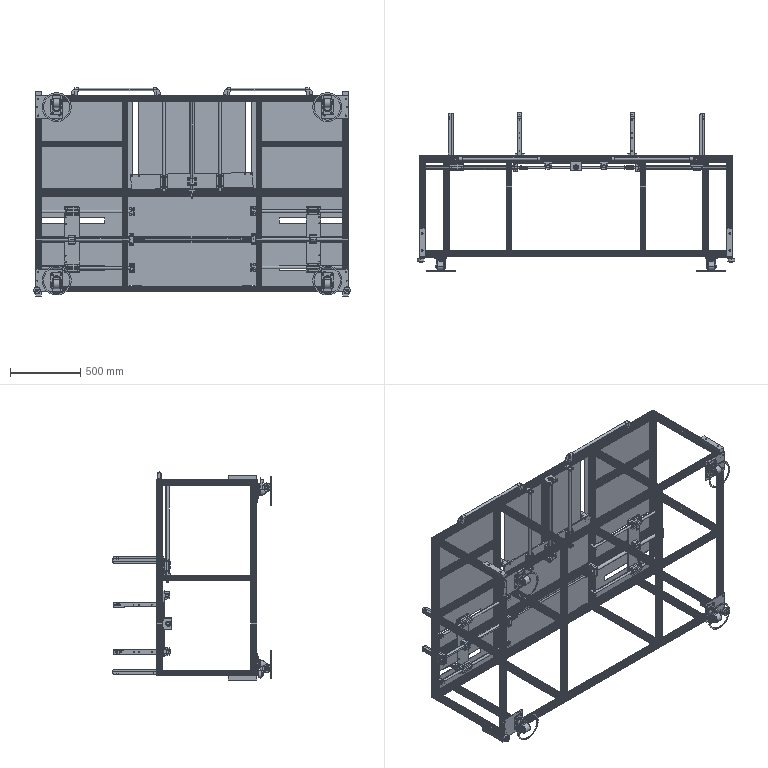Part | SolidWorks | features ReferencePattern 157, MirrorCompFeat 6, LocalLPattern 1 | 159 solids | 7866 faces | volume 40596234 mm3 | plane 4471 | cylinder 2375 | cone 630 | spline 366 | torus 24 | commonest cylinder face diameters 6 x443 9 x268 6.8 x172 5 x168 6.6 x160 20 x118